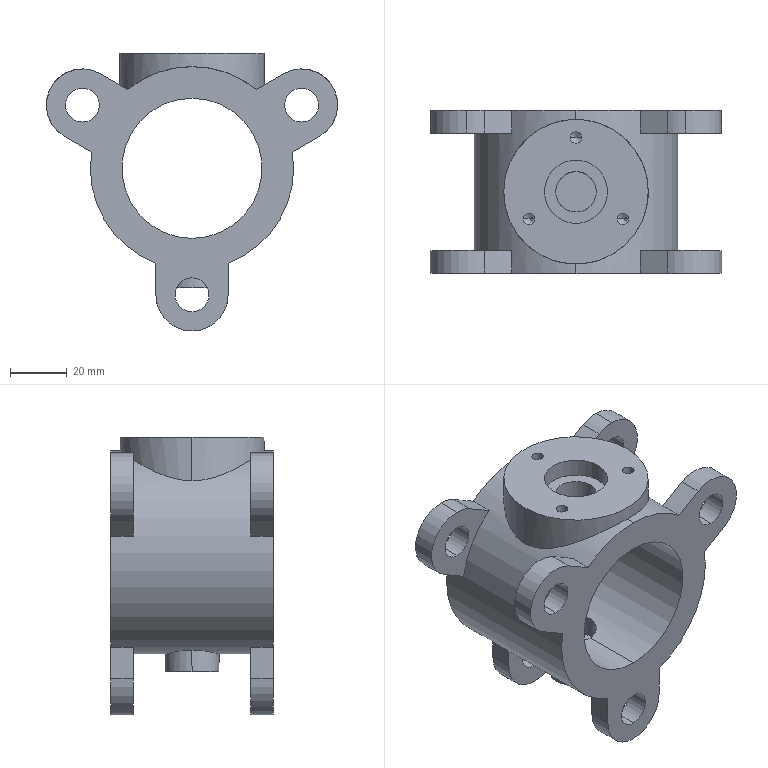Part | SolidWorks | features ICE 5, CirPattern 1, Extrusion 1, HoleWzd 1, MirrorPattern 1, RefAxis 1 | 1 solid | 71 faces | box 102.39 x 57.15 x 97.638 mm | volume 149520 mm3 | cylinder 41 | plane 24 | cone 6 | commonest cylinder face diameters 11.938 x12 25.4 x9 4.039 x6 14.275 x4 19.05 x2 22.225 x2